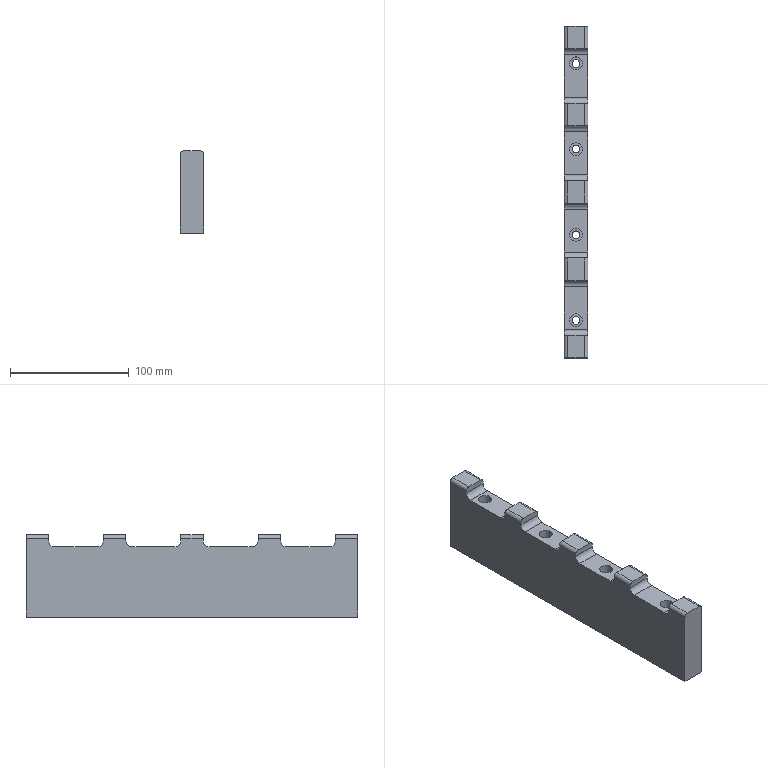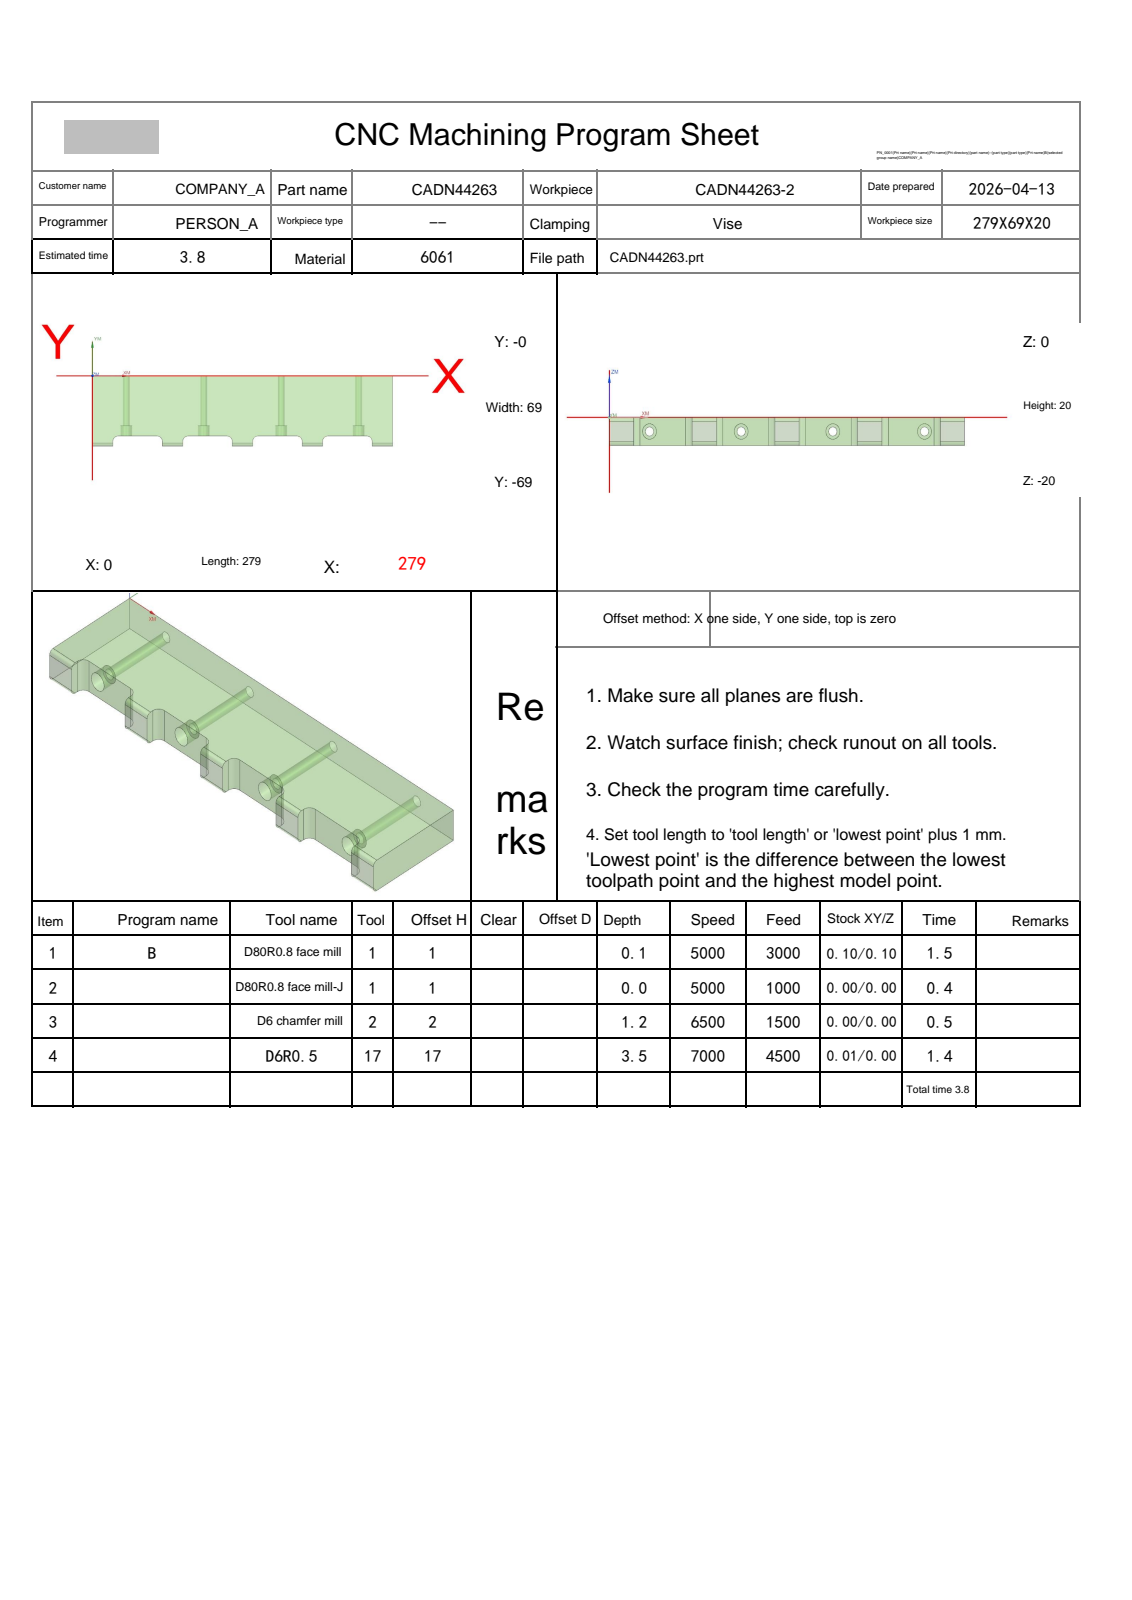NC program | NX | posted by the shop | part box 20 x 279 x 69 mm
Whole program:
%
O0001
(Machine time: 4.53 MIN)
(===Total Tool:3===)
(T1=D80R0.8 face mill D=80.  R=0.8  D-  H01 Z=0.    )
(T2=D6 chamfer mill   D=6.   R=0.   D-  H02 Z=-1.2  )
(T17=D6R0.5 D=6.   R=0.5  D-  H17 Z=-3.5  )
G80 G90 G17 G49 G40
G91 G28 Z0
M01
N1 T01 M06
(D80R0.8 face mill  D=80. R=0.8 H=01 ce=0.10 di=0.10)
G00 G90 G54 X-52.097 Y-34.5 M03 S5000
G43 H01 Z50.
M08
Z6.011
G01 Z4.011 F3000.
X-40.097
X319.097
X331.097
Z6.011
G00 X-52.097
Z5.522
G01 Z3.522
X-40.097
X319.097
X331.097
Z5.522
G00 X-52.097
Z5.033
G01 Z3.033
X-40.097
X319.097
X331.097
Z5.033
G00 X-52.097
Z4.544
G01 Z2.544
X-40.097
X319.097
X331.097
Z4.544
G00 Z50.
X-52.097
Z4.056
G01 Z2.056
X-40.097
X319.097
X331.097
Z4.056
G00 Z50.
X-52.097
Z3.567
G01 Z1.567
X-40.097
X319.097
X331.097
Z3.567
G00 Z50.
X-52.097
Z3.078
G01 Z1.078
X-40.097
X319.097
X331.097
Z3.078
G00 Z50.
X-52.097
Z2.589
G01 Z.589
X-40.097
X319.097
X331.097
Z2.589
G00 Z50.
X-52.097
Z2.1
G01 Z.1
X-40.097
X319.097
X331.097
Z2.1
G00 Z50.
G91 G28 Z0.0
M05
M09
G91 G28 Z0.0
M01
N2 T01 M06
(D80R0.8 face mill-J  D=80. R=0.8 H=01 ce=0.00 di=0.00)
G00 G90 G54 X-51.999 Y-34.5 M03 S5000
G43 H01 Z50.
M08
Z2.
G01 Z0.0 F1000.
X-39.999
X318.999
X330.999
Z2.
G00 Z50.
G91 G28 Z0.0
M05
M09
G91 G28 Z0.0
M01
N3 T02 M06
(D6 chamfer mill  D=6. R=0. H=02 ce=0.00 di=0.00)
G00 G90 G54 X64.072 Y-66.349 M03 S6500
G43 H02 Z50.
M08
Z2.801
G01 Z-1.199 F1500.
X64.034 Y-66.259
X64. Y-66.
Y-64.
G03 X60. Y-60. I-4. J0.0
G01 X24.
G03 X20. Y-64. I0.0 J-4.
G01 Y-66.
X19.997 Y-66.054
X20.027 Y-66.1
G03 X20.227 Y-66.386 I1.732 J1.
G01 Z.145
G00 Z10.
X129.072 Y-66.349
Z2.801
G01 Z-1.199
X129.034 Y-66.259
X129. Y-66.
Y-64.
G03 X125. Y-60. I-4. J0.0
G01 X89.
G03 X85. Y-64. I0.0 J-4.
G01 Y-66.
X84.997 Y-66.054
X85.027 Y-66.1
G03 X85.227 Y-66.386 I1.732 J1.
G01 Z.145
G00 Z10.
X193.773
Z.145
G01 Z-1.199
G03 X193.973 Y-66.1 I-1.532 J1.286
G01 X194.003 Y-66.054
X194. Y-66.
Y-64.
G03 X190. Y-60. I-4. J0.0
G01 X154.
G03 X150. Y-64. I0.0 J-4.
G01 Y-66.
X149.997 Y-66.054
X150.027 Y-66.1
G03 X150.227 Y-66.386 I1.732 J1.
G01 Z.145
G00 Z10.
X258.773
Z.145
G01 Z-1.199
G03 X258.973 Y-66.1 I-1.532 J1.286
G01 X259.003 Y-66.054
X259. Y-66.
Y-64.
G03 X255. Y-60. I-4. J0.0
G01 X219.
G03 X215. Y-64. I0.0 J-4.
G01 Y-66.
X214.997 Y-66.054
X215.027 Y-66.1
G03 X215.227 Y-66.386 I1.732 J1.
G01 Z.145
G00 Z10.
X-1.227
Z.145
G01 Z-1.199
G03 X-1.027 Y-66.1 I-1.532 J1.286
G01 X-.997 Y-66.054
X-1. Y-66.
Y0.0
G02 X0.0 Y1. I1. J0.0
G01 X279.
G02 X280. Y0.0 I0.0 J-1.
G01 Y-66.
X279.997 Y-66.054
X280.027 Y-66.1
G03 X280.227 Y-66.386 I1.732 J1.
G01 Z.145
G00 Z50.
G91 G28 Z0.0
M05
M09
G91 G28 Z0.0
M01
N4 T17 M06
(D6R0.5  D=6. R=0.5 H=17 ce=0.01 di=0.00)
G00 G90 G54 X285.345 Y-67.925 M03 S7000
G43 H17 Z14.8
M08
Z.493
G01 Z-.007 F4500.
X280.1 Y-68.533
X279. Y-68.738
X260.
G03 X259.218 Y-68.576 I-.782 J-1.81
X258.898 Y-68.602 I0.0 J-1.972
G01 X258.9 Y-68.67 Z-.015
G02 X260. Y-68.833 I-.342 J-6.077
G01 X279.
G03 X280.1 Y-68.642 I-.357 J5.306
G01 Y-68.755 Z-.023
X279. Y-68.91
X260.
X259.03 Y-68.74
X258.9 Y-68.731
Y-68.792 Z-.032
X260. Y-68.979
X279.
G02 X280.1 Y-68.813 I20.613 J-132.954
G01 Y-68.861 Z-.037
Y-68.876 Z-.042
X279. Y-69.053
X260.
X258.9 Y-68.85
X258.899 Y-68.898 Z-.049
Y-68.918 Z-.055
G03 X260. Y-69.128 I2.405 J9.652
G01 X279.
X280.1 Y-68.948
Y-69.007 Z-.062
Y-69.031 Z-.069
X279. Y-69.203
X260.
G02 X258.899 Y-68.996 I1.051 J8.641
G01 Y-69.042 Z-.077
Y-69.084 Z-.086
X260. Y-69.279
X279.
X280.1 Y-69.12
Y-69.155 Z-.095
Y-69.188 Z-.104
X279. Y-69.357
X260.
X258.9 Y-69.163
Y-69.196 Z-.114
Y-69.246 Z-.125
X260. Y-69.437
X279.
X279.053 Y-69.433
X280.1 Y-69.267
Y-69.311 Z-.137
Y-69.354 Z-.148
X279. Y-69.518
X260.
G02 X258.9 Y-69.339 I2.137 J16.607
G01 Y-69.386 Z-.161
Y-69.441 Z-.174
G03 X260. Y-69.599 I4.317 J26.016
G01 X279.
X280.1 Y-69.449
Y-69.503 Z-.188
X280.101 Y-69.546 Z-.203
G02 X279. Y-69.684 I-24.833 J193.175
G01 X260.
G02 X258.9 Y-69.541 I4.785 J41.204
G01 Y-69.595 Z-.219
Y-69.642 Z-.235
X260. Y-69.77
X279.
G02 X280.101 Y-69.644 I2.054 J-13.021
G01 Y-69.686 Z-.252
Y-69.727 Z-.269
G02 X279. Y-69.856 I-13.879 J113.455
G01 X260.
X258.9 Y-69.725
Y-69.772 Z-.288
Y-69.814 Z-.306
X260. Y-69.942
X279.
G02 X280.1 Y-69.814 I2.624 J-17.885
G01 Y-69.854 Z-.321
Y-69.883 Z-.337
G03 X279. Y-70.007 I.984 J-13.603
G01 X260.
G02 X258.9 Y-69.884 I3.105 J32.646
G01 Y-69.936 Z-.355
Y-69.97 Z-.374
G02 X260. Y-70.084 I-10.94 J-110.729
G01 X279.
G02 X280.1 Y-69.967 I1.926 J-12.88
G01 Y-70.032 Z-.396
Y-70.067 Z-.418
G03 X279. Y-70.169 I.819 J-14.766
G01 X260.
G03 X258.9 Y-70.066 I-2.92 J-25.349
G01 Y-70.119 Z-.442
Y-70.16 Z-.465
X259.082 Y-70.162
X260. Y-70.253
X279.
G02 X280.1 Y-70.161 I1.249 J-8.298
G01 Y-70.202 Z-.49
Y-70.242 Z-.515
G03 X279. Y-70.337 I.124 J-7.861
G01 X260.
X259.082 Y-70.243
X258.9 Y-70.24
Y-70.285 Z-.54
Y-70.324 Z-.566
X259.082 Y-70.327
X260. Y-70.418
X279.
G02 X280.1 Y-70.326 I1.273 J-8.566
G01 Y-70.368 Z-.591
Y-70.409 Z-.617
X279.742 Y-70.41
G02 X279. Y-70.495 I-.89 J4.508
G01 X260.
G03 X258.9 Y-70.407 I-1.859 J-16.484
G01 Y-70.453 Z-.644
Y-70.489 Z-.67
X259.082 Y-70.491
X260. Y-70.569
X279.
G02 X280.1 Y-70.49 I1.178 J-8.684
G01 Y-70.537 Z-.699
Y-70.563 Z-.729
G03 X279. Y-70.648 I.05 J-7.856
G01 X260.
X259.082 Y-70.564
X258.9 Y-70.562
Y-70.614 Z-.759
Y-70.638 Z-.79
X259.082 Y-70.64
X260. Y-70.725
X279.
G02 X280.1 Y-70.639 I1.177 J-8.027
G01 Y-70.687 Z-.822
Y-70.718 Z-.853
G03 X279. Y-70.8 I.177 J-9.805
G01 X260.
G03 X258.9 Y-70.716 I-1.551 J-13.131
G01 Y-70.763 Z-.886
Y-70.798 Z-.919
G02 X260. Y-70.874 I-.529 J-15.689
G01 X279.
G02 X280.1 Y-70.8 I1.318 J-11.377
G01 Y-70.841 Z-.952
Y-70.876 Z-.986
G03 X279. Y-70.945 I.124 J-10.694
G01 X260.
G03 X258.9 Y-70.874 I-1.437 J-13.654
G01 Y-70.921 Z-1.021
Y-70.951 Z-1.056
X259.082 Y-70.954
X260. Y-71.015
X279.
G02 X280.101 Y-70.953 I1.228 J-11.902
G01 Y-70.989 Z-1.092
Y-71.021 Z-1.128
G03 X279. Y-71.084 I.035 J-10.406
G01 X260.
G03 X258.9 Y-71.02 I-1.26 J-12.225
G01 Y-71.054 Z-1.165
Y-71.083 Z-1.202
X259.427 Y-71.096
G03 X260. Y-71.15 I.614 J3.478
G01 X279.
G02 X280.1 Y-71.085 I1.194 J-10.827
G01 Y-71.118 Z-1.24
Y-71.149 Z-1.278
G03 X279. Y-71.214 I.089 J-10.915
G01 X260.
G02 X259.427 Y-71.161 I.105 J4.261
G01 X258.9 Y-71.148
Y-71.183 Z-1.316
Y-71.212 Z-1.355
G02 X260. Y-71.276 I-.313 J-14.825
G01 X279.
G02 X280.1 Y-71.213 I1.165 J-10.805
G01 X280.101 Y-71.25 Z-1.395
Y-71.279 Z-1.434
G03 X279. Y-71.336 I.103 J-12.677
G01 X260.
G03 X258.9 Y-71.277 I-1.704 J-21.57
G01 Y-71.31 Z-1.475
Y-71.339 Z-1.516
G02 X260. Y-71.393 I-.086 J-12.93
G01 X279.
G02 X280.08 Y-71.34 I1.08 J-11.01
G01 X280.101
Y-71.367 Z-1.557
Y-71.391 Z-1.598
X280.085
G03 X279. Y-71.448 I0.0 J-10.303
G01 X260.
X259.427 Y-71.4
X258.9 Y-71.39
Y-71.418 Z-1.641
Y-71.441 Z-1.683
X259.427 Y-71.452
G03 X260. Y-71.501 I.616 J3.827
G01 X279.
X279.053 Y-71.5
X279.727 Y-71.446
G02 X279.938 Y-71.438 I.211 J-2.639
G01 X280.1 Y-71.443
Y-71.47 Z-1.726
Y-71.496 Z-1.769
X280.052
G03 X279. Y-71.552 I0.0 J-9.962
G01 X260.
G02 X259.427 Y-71.505 I.274 J6.879
G01 X258.9 Y-71.496
Y-71.523 Z-1.812
Y-71.547 Z-1.856
G02 X260. Y-71.6 I-.079 J-13.17
G01 X279.
G02 X279.98 Y-71.548 I.98 J-9.242
G01 X280.101 Y-71.549
Y-71.573 Z-1.9
Y-71.597 Z-1.945
X279.972 Y-71.596
G03 X279. Y-71.645 I0.0 J-9.55
G01 X260.
G03 X258.9 Y-71.596 I-1.189 J-14.048
G01 Y-71.618 Z-1.99
Y-71.635 Z-2.035
X259.427 Y-71.644
G03 X260. Y-71.689 I.669 J4.914
G01 X279.
G02 X280.09 Y-71.636 I1.09 J-11.268
G01 X280.101
Y-71.657 Z-2.08
Y-71.675 Z-2.126
X280.025
G03 X279. Y-71.729 I0.0 J-9.733
G01 X260.
G02 X259.427 Y-71.683 I.123 J5.164
G01 X258.9 Y-71.674
Y-71.695 Z-2.172
Y-71.712 Z-2.218
X259.427 Y-71.722
G03 X260. Y-71.767 I.648 J4.552
G01 X279.
G02 X279.983 Y-71.713 I.983 J-8.893
G01 X280.101 Y-71.714
Y-71.734 Z-2.265
Y-71.752 Z-2.312
X279.959 Y-71.751
G03 X279. Y-71.802 I0.0 J-9.028
G01 X260.
G02 X259.427 Y-71.76 I.241 J7.253
G01 X258.9 Y-71.751
Y-71.771 Z-2.359
Y-71.789 Z-2.406
G02 X260. Y-71.835 I-.203 J-18.176
G01 X279.
G02 X279.96 Y-71.79 I.96 J-10.236
G01 X280.102 Y-71.791
X280.101 Y-71.807 Z-2.454
X280.1 Y-71.817 Z-2.502
X280.092
G03 X279. Y-71.865 I0.0 J-12.564
G01 X260.
X259.427 Y-71.824
X258.9 Y-71.817
X258.898 Y-71.833 Z-2.55
X258.896 Y-71.846 Z-2.598
X259.427 Y-71.85
X260. Y-71.892
X279.
G02 X280.038 Y-71.842 I1.038 J-10.908
G01 X280.1 Y-71.843
X280.097 Y-71.854 Z-2.646
X280.095 Y-71.866 Z-2.695
G03 X279. Y-71.916 I.01 J-12.239
G01 X260.
X259.427 Y-71.875
X258.896 Y-71.872
Y-71.885 Z-2.744
X258.895 Y-71.898 Z-2.792
X259.427 Y-71.901
X260. Y-71.938
X279.
G02 X280.096 Y-71.89 I1.259 J-16.152
G01 X280.097 Y-71.901 Z-2.841
Y-71.913 Z-2.891
G03 X279. Y-71.957 I.411 J-24.268
G01 X260.
G03 X258.995 Y-71.922 I-1.005 J-14.556
G01 X258.895
Y-71.931 Z-2.94
Y-71.942 Z-2.989
X259.028 Y-71.941
G02 X260. Y-71.973 I0.0 J-15.169
G01 X279.
G02 X280.098 Y-71.935 I1.532 J-29.007
G01 X280.099 Y-71.945 Z-3.039
Y-71.955 Z-3.088
X279. Y-71.986
X260.
G03 X259.128 Y-71.96 I-.872 J-14.727
X258.895 Y-71.962 I0.0 J-14.753
G01 X258.905 Y-71.976 Z-3.188
G02 X259.203 Y-71.973 I.298 J-13.938
X260. Y-71.996 I0.0 J-13.941
G01 X279.
X279.053 Y-71.993
X280.1 Y-71.973
X280.101 Y-71.979 Z-3.227
Y-71.983 Z-3.266
X279.053 Y-71.998
X279. Y-72.002
X260.
G03 X259.208 Y-71.983 I-.792 J-16.081
X258.905 Y-71.986 I0.0 J-16.1
G01 Y-71.995 Z-3.344
G02 X259.211 Y-71.992 I.306 J-22.158
X260. Y-72.007 I0.0 J-22.16
G01 X279.
X280.101 Y-71.993
X280.102 Y-71.999 Z-3.383
Y-72.003 Z-3.422
X279. Y-72.009
X260.
X258.905 Y-72.004
Y-72.009 Z-3.5
X280.102
G00 Z14.8
X219.775 Y-69.035
Z.493
G01 Z-.007
X215.1 Y-68.532
X214.882 Y-68.533
X214. Y-68.738
X195.
X194.118 Y-68.533
X193.91 Y-68.573
X193.903 Y-68.638 Z-.011
X193.902 Y-68.651 Z-.015
X194.81 Y-68.807
X195. Y-68.833
X214.
G02 X215.1 Y-68.64 I11.736 J-63.511
G01 Y-68.721 Z-.019
Y-68.752 Z-.023
X214. Y-68.91
X195.
X193.898 Y-68.732
X193.9 Y-68.79 Z-.032
X194.113 Y-68.818
X195. Y-68.979
X214.
X214.882 Y-68.813
X215.1 Y-68.812
Y-68.861 Z-.037
Y-68.875 Z-.042
X214.882 Y-68.877
X214. Y-69.053
X195.
X194.109 Y-68.893
X193.9 Y-68.847
Y-68.898 Z-.049
Y-68.915 Z-.055
X194.096 Y-68.955
X195. Y-69.128
X214.
X214.882 Y-68.951
X215.1 Y-68.948
Y-69.007 Z-.062
Y-69.031 Z-.069
X214. Y-69.203
X195.
G02 X193.9 Y-68.992 I1.243 J9.475
G01 Y-69.043 Z-.077
Y-69.081 Z-.086
X194.066 Y-69.107
X195. Y-69.279
X214.
X215.1 Y-69.12
Y-69.155 Z-.095
Y-69.189 Z-.104
X214. Y-69.357
X195.
X193.899 Y-69.164
Y-69.196 Z-.114
Y-69.248 Z-.125
X195. Y-69.437
X214.
X215.1 Y-69.268
Y-69.311 Z-.137
Y-69.355 Z-.148
X214. Y-69.518
X195.
X194.81 Y-69.503
X193.9 Y-69.342
Y-69.386 Z-.161
Y-69.441 Z-.174
X195. Y-69.599
X214.
X215.1 Y-69.45
Y-69.503 Z-.188
Y-69.546 Z-.203
X214.882 Y-69.55
X214. Y-69.684
X195.
X194.118 Y-69.55
X193.899 Y-69.543
X193.9 Y-69.596 Z-.219
Y-69.643 Z-.235
X195. Y-69.77
X214.
X214.882 Y-69.645
X215.1 Y-69.643
Y-69.686 Z-.252
Y-69.726 Z-.269
X214.882 Y-69.728
X214. Y-69.856
X195.
X193.9 Y-69.726
Y-69.772 Z-.288
Y-69.813 Z-.306
X194.118 Y-69.815
X195. Y-69.942
X214.
X214.882 Y-69.817
X215.1 Y-69.814
Y-69.854 Z-.321
Y-69.884 Z-.337
G03 X214. Y-70.007 I11.318 J-105.893
G01 X195.
X194.118 Y-69.884
X193.9 Y-69.882
Y-69.936 Z-.355
Y-69.966 Z-.374
X195. Y-70.084
X214.
X214.882 Y-69.978
X215.1 Y-69.97
Y-70.033 Z-.396
Y-70.067 Z-.418
X214.882 Y-70.072
X214. Y-70.169
X195.
X193.9 Y-70.065
Y-70.119 Z-.442
Y-70.16 Z-.465
X194.118 Y-70.162
X195. Y-70.253
X214.
X214.882 Y-70.162
X215.1 Y-70.16
Y-70.202 Z-.49
Y-70.241 Z-.515
X214.882 Y-70.243
X214. Y-70.337
X195.
G02 X194.292 Y-70.247 I.042 J3.181
G01 X193.9 Y-70.241
Y-70.285 Z-.54
Y-70.325 Z-.566
X194.118 Y-70.327
X195. Y-70.418
X214.
X214.882 Y-70.327
X215.1 Y-70.325
Y-70.368 Z-.591
Y-70.408 Z-.617
X214.882 Y-70.41
X214. Y-70.495
X195.
X193.9 Y-70.408
Y-70.453 Z-.644
Y-70.49 Z-.67
X194.118 Y-70.491
X195. Y-70.569
X214.
G02 X215.1 Y-70.49 I1.409 J-11.774
G01 Y-70.537 Z-.699
Y-70.563 Z-.729
G03 X214. Y-70.648 I.234 J-10.139
G01 X195.
X194.118 Y-70.564
X193.9 Y-70.563
Y-70.614 Z-.759
Y-70.638 Z-.79
X194.118 Y-70.64
X195. Y-70.725
X214.
G02 X215.1 Y-70.638 I1.321 J-9.774
G01 Y-70.687 Z-.822
Y-70.717 Z-.853
X214.955 Y-70.709
X214.821 Y-70.716
X214. Y-70.8
X195.
X194.118 Y-70.719
X193.9 Y-70.717
Y-70.763 Z-.886
Y-70.798 Z-.919
X194.118 Y-70.8
X195. Y-70.874
X214.
X214.536 Y-70.823
X214.62 Y-70.814
X215.1 Y-70.798
Y-70.841 Z-.952
Y-70.875 Z-.986
X214.882 Y-70.877
X214. Y-70.945
X195.
X194.118 Y-70.877
X193.9 Y-70.875
Y-70.919 Z-1.021
Y-70.952 Z-1.056
X194.118 Y-70.954
X195. Y-71.015
X214.
X214.882 Y-70.954
X215.1 Y-70.952
Y-70.989 Z-1.092
Y-71.021 Z-1.128
G03 X214. Y-71.084 I.106 J-11.464
G01 X195.
G03 X193.9 Y-71.021 I-1.206 J-11.401
G01 Y-71.054 Z-1.165
Y-71.084 Z-1.202
X194.464 Y-71.1
G03 X195. Y-71.15 I.558 J3.082
G01 X214.
G03 X214.536 Y-71.1 I-.021 J3.132
G01 X215.1 Y-71.084
Y-71.118 Z-1.24
Y-71.148 Z-1.278
G03 X214. Y-71.214 I.353 J-15.186
G01 X195.
G03 X193.9 Y-71.148 I-1.453 J-15.12
G01 Y-71.183 Z-1.316
Y-71.212 Z-1.355
G02 X195. Y-71.276 I-.249 J-13.86
G01 X214.
G02 X215.1 Y-71.212 I1.349 J-13.797
G01 Y-71.25 Z-1.395
Y-71.277 Z-1.434
G03 X214. Y-71.336 I.651 J-22.793
G01 X195.
G03 X193.9 Y-71.277 I-1.752 J-22.735
G01 Y-71.31 Z-1.475
Y-71.339 Z-1.516
G02 X195. Y-71.393 I-.06 J-12.531
G01 X214.
G02 X215.1 Y-71.339 I1.16 J-12.478
G01 Y-71.367 Z-1.557
Y-71.39 Z-1.598
G03 X214. Y-71.448 I.169 J-13.623
G01 X195.
G03 X193.9 Y-71.39 I-1.269 J-13.564
G01 Y-71.418 Z-1.641
Y-71.442 Z-1.683
X194.464 Y-71.455
G03 X195. Y-71.501 I.55 J3.271
G01 X214.
G03 X214.536 Y-71.455 I-.02 J3.386
G01 X215.1 Y-71.442
Y-71.47 Z-1.726
Y-71.496 Z-1.769
G03 X214. Y-71.552 I.175 J-14.347
G01 X195.
G03 X193.9 Y-71.496 I-1.275 J-14.292
G01 Y-71.523 Z-1.812
Y-71.548 Z-1.856
G02 X195. Y-71.6 I-.069 J-13.12
G01 X214.
G02 X215.1 Y-71.548 I1.169 J-13.068
G01 Y-71.573 Z-1.9
Y-71.596 Z-1.945
G03 X214. Y-71.645 I.103 J-14.555
G01 X195.
G03 X193.9 Y-71.596 I-1.203 J-14.506
G01 Y-71.618 Z-1.99
Y-71.635 Z-2.035
X194.464 Y-71.647
G03 X195. Y-71.689 I.605 J4.327
G01 X214.
G03 X214.536 Y-71.647 I-.069 J4.369
G01 X215.1 Y-71.635
Y-71.657 Z-2.08
Y-71.674 Z-2.126
X214.536 Y-71.686
G02 X214. Y-71.729 I-.622 J4.418
G01 X195.
G02 X194.464 Y-71.686 I.086 J4.461
G01 X193.9 Y-71.674
Y-71.695 Z-2.172
Y-71.713 Z-2.218
X194.464 Y-71.725
G03 X195. Y-71.767 I.59 J4.056
G01 X214.
G03 X214.536 Y-71.725 I-.054 J4.098
G01 X215.1 Y-71.713
Y-71.734 Z-2.265
Y-71.751 Z-2.312
X214.536 Y-71.761
G02 X214. Y-71.802 I-.689 J5.53
G01 X195.
G02 X194.464 Y-71.763 I.182 J6.232
G01 X193.9 Y-71.751
Y-71.771 Z-2.359
Y-71.79 Z-2.406
X194.464 Y-71.8
G03 X195. Y-71.835 I.669 J6.159
G01 X214.
X214.19 Y-71.828
G02 X214.861 Y-71.784 I.671 J-5.154
X215.1 Y-71.79 I0.0 J-5.198
G01 Y-71.807 Z-2.454
Y-71.816 Z-2.502
G03 X214. Y-71.865 I.147 J-15.87
G01 X195.
G03 X193.9 Y-71.818 I-1.19 J-15.04
G01 X193.898 Y-71.833 Z-2.55
X193.897 Y-71.846 Z-2.598
X193.953
G02 X195. Y-71.892 I0.0 J-12.019
G01 X214.
G02 X215.103 Y-71.843 I1.135 J-13.09
G01 Y-71.854 Z-2.646
Y-71.866 Z-2.695
G03 X214. Y-71.916 I.267 J-18.114
G01 X195.
G02 X194.464 Y-71.878 I.19 J6.461
G01 X193.897 Y-71.872
Y-71.885 Z-2.744
Y-71.898 Z-2.792
X194.464 Y-71.903
X195. Y-71.938
X214.
G02 X215.103 Y-71.89 I1.534 J-22.69
G01 Y-71.901 Z-2.841
Y-71.914 Z-2.891
G03 X214. Y-71.957 I.475 J-26.586
G01 X195.
G03 X194.065 Y-71.923 I-.935 J-13.098
G01 X193.897 Y-71.924
Y-71.931 Z-2.94
X193.896 Y-71.943 Z-2.989
X194.071 Y-71.942
G02 X195. Y-71.973 I0.0 J-14.242
G01 X214.
G02 X215.103 Y-71.935 I1.619 J-31.516
G01 X215.104 Y-71.944 Z-3.039
Y-71.955 Z-3.088
X214.19 Y-71.976
X214. Y-71.986
X195.
G03 X194.142 Y-71.96 I-.858 J-14.468
X193.896 Y-71.962 I0.0 J-14.494
G01 Y-71.966 Z-3.138
Y-71.976 Z-3.188
X194.81 Y-71.984
X195. Y-71.996
X214.
X214.19 Y-71.984
X215.104 Y-71.972
Y-71.979 Z-3.227
Y-71.982 Z-3.266
X214.19 Y-71.991
X214. Y-72.002
X195.
X194.81 Y-71.991
X193.896 Y-71.985
Y-71.994 Z-3.344
X194.81 Y-71.998
X195. Y-72.007
X214.
X214.19 Y-71.998
X215.104 Y-71.992
Y-71.998 Z-3.383
Y-72.003 Z-3.422
X214.19 Y-72.005
X214. Y-72.009
X195.
X194.81 Y-72.005
X193.896 Y-72.003
Y-72.009 Z-3.5
X215.104
G00 Z14.8
X154.771 Y-69.038
Z.493
G01 Z-.007
X150.1 Y-68.532
X149.884
X149. Y-68.738
X130.
X129.116 Y-68.532
X128.91 Y-68.572
X128.903 Y-68.638 Z-.011
X128.902 Y-68.651 Z-.015
G02 X130. Y-68.833 I-3.049 J-21.763
G01 X149.
G02 X150.1 Y-68.64 I11.734 J-63.449
G01 Y-68.721 Z-.019
Y-68.753 Z-.023
X149. Y-68.91
X130.
X128.898 Y-68.732
X128.9 Y-68.79 Z-.032
X129.111 Y-68.818
X130. Y-68.979
X149.
X149.884 Y-68.813
X150.1 Y-68.812
Y-68.861 Z-.037
Y-68.874 Z-.042
X149.884 Y-68.876
X149. Y-69.053
X130.
X129.108 Y-68.892
X128.9 Y-68.848
Y-68.898 Z-.049
Y-68.916 Z-.055
X129.095 Y-68.955
X130. Y-69.128
X149.
X149.884 Y-68.95
X150.1 Y-68.948
Y-69.007 Z-.062
Y-69.031 Z-.069
X149. Y-69.203
X130.
G02 X128.9 Y-68.994 I.939 J7.967
G01 Y-69.042 Z-.077
Y-69.084 Z-.086
X129.064 Y-69.106
X130. Y-69.279
X149.
X150.1 Y-69.119
Y-69.155 Z-.095
Y-69.189 Z-.104
X149. Y-69.357
X130.
X128.899 Y-69.164
Y-69.196 Z-.114
Y-69.248 Z-.125
X130. Y-69.437
X149.
X150.1 Y-69.267
Y-69.311 Z-.137
Y-69.355 Z-.148
X149. Y-69.518
X130.
X129.808 Y-69.503
X128.9 Y-69.342
Y-69.386 Z-.161
Y-69.441 Z-.174
X130. Y-69.599
X149.
X150.1 Y-69.45
Y-69.503 Z-.188
Y-69.546 Z-.203
X149.884 Y-69.55
X149. Y-69.684
X130.
X129.116 Y-69.55
X128.9 Y-69.543
Y-69.596 Z-.219
Y-69.643 Z-.235
X130. Y-69.77
X149.
X149.884 Y-69.645
X150.1 Y-69.643
Y-69.686 Z-.252
Y-69.726 Z-.269
X149.884 Y-69.728
X149. Y-69.856
X130.
X128.9 Y-69.726
Y-69.772 Z-.288
Y-69.813 Z-.306
X129.116 Y-69.815
X130. Y-69.942
X149.
X149.884 Y-69.817
X150.1 Y-69.814
Y-69.854 Z-.321
Y-69.884 Z-.337
G03 X149. Y-70.007 I11.328 J-105.982
G01 X130.
X129.116 Y-69.884
X128.9 Y-69.882
Y-69.936 Z-.355
Y-69.966 Z-.374
X130. Y-70.084
X149.
X149.884 Y-69.978
X150.1 Y-69.97
Y-70.032 Z-.396
Y-70.067 Z-.418
X149.884 Y-70.072
X149. Y-70.169
X130.
X128.9 Y-70.066
Y-70.119 Z-.442
Y-70.16 Z-.465
X129.116 Y-70.162
X130. Y-70.253
X149.
X149.884 Y-70.162
X150.1 Y-70.16
Y-70.202 Z-.49
Y-70.241 Z-.515
X149.884 Y-70.243
X149. Y-70.337
X130.
G02 X129.291 Y-70.247 I.043 J3.197
G01 X128.9 Y-70.241
Y-70.285 Z-.54
Y-70.325 Z-.566
X129.116 Y-70.327
X130. Y-70.418
X149.
X149.884 Y-70.327
X150.1 Y-70.325
Y-70.368 Z-.591
Y-70.408 Z-.617
X149.884 Y-70.41
X149. Y-70.495
X130.
X128.9 Y-70.408
Y-70.453 Z-.644
Y-70.489 Z-.67
X129.116 Y-70.491
X130. Y-70.569
X149.
G02 X150.1 Y-70.489 I1.413 J-11.804
G01 Y-70.537 Z-.699
Y-70.562 Z-.729
G03 X149. Y-70.648 I.236 J-10.157
G01 X130.
X129.116 Y-70.564
X128.9 Y-70.562
Y-70.614 Z-.759
Y-70.638 Z-.79
X129.116 Y-70.64
X130. Y-70.725
X149.
G02 X150.1 Y-70.638 I1.324 J-9.805
G01 Y-70.687 Z-.822
Y-70.717 Z-.853
X149.956 Y-70.711
X149.784 Y-70.72
X149. Y-70.8
X130.
X129.116 Y-70.719
X128.9 Y-70.717
Y-70.763 Z-.886
Y-70.798 Z-.919
X129.116 Y-70.8
X130. Y-70.874
X149.
X149.538 Y-70.822
X149.626 Y-70.813
X150.1 Y-70.798
Y-70.841 Z-.952
Y-70.875 Z-.986
X149.884 Y-70.877
X149. Y-70.945
X130.
X129.116 Y-70.877
X128.9 Y-70.875
Y-70.921 Z-1.021
Y-70.952 Z-1.056
X129.116 Y-70.954
X130. Y-71.015
X149.
X149.884 Y-70.954
X150.1 Y-70.952
Y-70.989 Z-1.092
Y-71.02 Z-1.128
G03 X149. Y-71.084 I.108 J-11.494
G01 X130.
G03 X128.9 Y-71.02 I-1.208 J-11.431
G01 Y-71.054 Z-1.165
Y-71.084 Z-1.202
X129.462 Y-71.1
G03 X130. Y-71.15 I.559 J3.085
G01 X149.
G03 X149.538 Y-71.1 I-.021 J3.135
G01 X150.1 Y-71.084
Y-71.118 Z-1.24
Y-71.148 Z-1.278
G03 X149. Y-71.214 I.356 J-15.218
G01 X130.
G03 X128.9 Y-71.148 I-1.456 J-15.152
G01 Y-71.183 Z-1.316
Y-71.212 Z-1.355
G02 X130. Y-71.276 I-.253 J-13.932
G01 X149.
G02 X150.1 Y-71.212 I1.353 J-13.869
G01 Y-71.25 Z-1.395
Y-71.278 Z-1.434
G03 X149. Y-71.336 I.659 J-22.96
G01 X130.
G03 X128.9 Y-71.278 I-1.759 J-22.9
G01 Y-71.31 Z-1.475
Y-71.339 Z-1.516
G02 X130. Y-71.393 I-.061 J-12.531
G01 X149.
G02 X150.1 Y-71.339 I1.161 J-12.477
G01 Y-71.367 Z-1.557
Y-71.39 Z-1.598
G03 X149. Y-71.448 I.174 J-13.705
G01 X130.
G03 X128.9 Y-71.39 I-1.274 J-13.647
G01 Y-71.418 Z-1.641
Y-71.442 Z-1.683
X129.462 Y-71.455
G03 X130. Y-71.501 I.551 J3.272
G01 X149.
G03 X149.538 Y-71.455 I-.017 J3.362
G01 X150.1 Y-71.442
Y-71.47 Z-1.726
Y-71.496 Z-1.769
G03 X149. Y-71.552 I.189 J-14.504
G01 X130.
G03 X128.9 Y-71.496 I-1.288 J-14.447
G01 Y-71.523 Z-1.812
Y-71.548 Z-1.856
G02 X130. Y-71.6 I-.07 J-13.129
G01 X149.
G02 X150.1 Y-71.548 I1.17 J-13.077
G01 Y-71.573 Z-1.9
Y-71.596 Z-1.945
G03 X149. Y-71.645 I.111 J-14.702
G01 X130.
G03 X128.9 Y-71.596 I-1.211 J-14.652
G01 Y-71.618 Z-1.99
Y-71.635 Z-2.035
X129.462 Y-71.647
G03 X130. Y-71.689 I.608 J4.36
G01 X149.
G03 X149.538 Y-71.647 I-.07 J4.402
G01 X150.1 Y-71.635
Y-71.657 Z-2.08
Y-71.674 Z-2.126
X149.538 Y-71.686
G02 X149. Y-71.729 I-.624 J4.432
G01 X130.
G02 X129.462 Y-71.686 I.086 J4.475
G01 X128.9 Y-71.674
Y-71.695 Z-2.172
Y-71.713 Z-2.218
X129.462 Y-71.724
G03 X130. Y-71.767 I.594 J4.092
G01 X149.
G03 X149.538 Y-71.724 I-.056 J4.134
G01 X150.1 Y-71.713
Y-71.734 Z-2.265
Y-71.751 Z-2.312
X149.538 Y-71.761
G02 X149. Y-71.802 I-.691 J5.54
G01 X130.
G02 X129.462 Y-71.763 I.184 J6.258
G01 X128.9 Y-71.751
Y-71.771 Z-2.359
Y-71.79 Z-2.406
X129.462 Y-71.8
G03 X130. Y-71.835 I.668 J6.118
G01 X149.
X149.192 Y-71.828
G02 X149.86 Y-71.784 I.669 J-5.13
X150.1 Y-71.79 I0.0 J-5.173
G01 Y-71.807 Z-2.454
Y-71.816 Z-2.502
G03 X149. Y-71.865 I.142 J-15.739
G01 X130.
G03 X128.9 Y-71.818 I-1.186 J-14.917
G01 Y-71.833 Z-2.55
Y-71.846 Z-2.598
X128.957
G02 X130. Y-71.892 I0.0 J-11.927
G01 X149.
G02 X150.1 Y-71.843 I1.132 J-13.003
G01 Y-71.854 Z-2.646
Y-71.866 Z-2.695
G03 X149. Y-71.916 I.261 J-17.894
G01 X130.
G02 X129.462 Y-71.878 I.199 J6.597
G01 X128.9 Y-71.872
Y-71.885 Z-2.744
Y-71.898 Z-2.792
X129.462 Y-71.903
G03 X130. Y-71.938 I.695 J6.615
G01 X149.
G02 X150.1 Y-71.89 I1.541 J-22.828
G01 Y-71.902 Z-2.841
Y-71.914 Z-2.891
X149.884 Y-71.918
X149. Y-71.957
X130.
G03 X129.014 Y-71.922 I-.986 J-14.218
G01 X128.901 Y-71.923
X128.9 Y-71.937 Z-2.94
Y-71.943 Z-2.989
X129.072 Y-71.942
G02 X130. Y-71.973 I0.0 J-14.315
G01 X149.
X149.884 Y-71.939
X150.1 Y-71.935
Y-71.945 Z-3.039
Y-71.955 Z-3.088
X149.192 Y-71.975
X149. Y-71.986
X130.
G03 X129.112 Y-71.96 I-.888 J-15.263
X128.9 Y-71.961 I0.0 J-15.289
G01 Y-71.971 Z-3.138
Y-71.975 Z-3.188
X129.808 Y-71.984
X130. Y-71.996
X149.
X149.192 Y-71.984
X150.1 Y-71.971
Y-71.979 Z-3.227
Y-71.982 Z-3.266
X149.192 Y-71.991
X149. Y-72.002
X130.
X129.808 Y-71.99
X128.9 Y-71.986
X128.905 Y-71.995 Z-3.344
X128.911 Y-71.993
X129.808 Y-71.997
X130. Y-72.007
X149.
X149.192 Y-71.997
X150.089 Y-71.992
X150.1 Y-71.994
X150.095 Y-72.002 Z-3.422
X149.192 Y-72.004
X149. Y-72.009
X130.
X129.808 Y-72.004
X128.905 Y-72.003
Y-72.01 Z-3.5
X150.095
G00 Z14.8
X89.775 Y-69.035
Z.493
G01 Z-.007
X85.1 Y-68.532
X84.882 Y-68.533
X84. Y-68.738
X65.
X64.118 Y-68.533
X63.91 Y-68.573
X63.903 Y-68.638 Z-.011
X63.902 Y-68.651 Z-.015
X64.81 Y-68.807
X65. Y-68.833
X84.
G02 X85.1 Y-68.64 I11.736 J-63.511
G01 Y-68.721 Z-.019
Y-68.752 Z-.023
X84. Y-68.91
X65.
X63.898 Y-68.732
X63.9 Y-68.79 Z-.032
X64.113 Y-68.818
X65. Y-68.979
X84.
X84.882 Y-68.813
X85.1 Y-68.812
Y-68.861 Z-.037
Y-68.875 Z-.042
X84.882 Y-68.877
X84. Y-69.053
X65.
X64.109 Y-68.893
X63.9 Y-68.847
Y-68.898 Z-.049
Y-68.915 Z-.055
X64.096 Y-68.955
X65. Y-69.128
X84.
X84.882 Y-68.951
X85.1 Y-68.948
Y-69.007 Z-.062
Y-69.031 Z-.069
X84. Y-69.203
X65.
G02 X63.9 Y-68.992 I1.243 J9.475
G01 Y-69.043 Z-.077
Y-69.081 Z-.086
X64.066 Y-69.107
X65. Y-69.279
X84.
X85.1 Y-69.12
Y-69.155 Z-.095
Y-69.189 Z-.104
X84. Y-69.357
X65.
X63.899 Y-69.164
Y-69.196 Z-.114
Y-69.248 Z-.125
X65. Y-69.437
X84.
X85.1 Y-69.268
Y-69.311 Z-.137
Y-69.355 Z-.148
X84. Y-69.518
X65.
X64.81 Y-69.503
X63.9 Y-69.342
Y-69.386 Z-.161
Y-69.441 Z-.174
X65. Y-69.599
X84.
X85.1 Y-69.45
Y-69.503 Z-.188
Y-69.546 Z-.203
X84.882 Y-69.55
X84. Y-69.684
X65.
X64.118 Y-69.55
X63.899 Y-69.543
X63.9 Y-69.596 Z-.219
Y-69.643 Z-.235
X65. Y-69.77
X84.
X84.882 Y-69.645
X85.1 Y-69.643
Y-69.686 Z-.252
Y-69.726 Z-.269
X84.882 Y-69.728
X84. Y-69.856
X65.
X63.9 Y-69.726
Y-69.772 Z-.288
Y-69.813 Z-.306
X64.118 Y-69.815
X65. Y-69.942
X84.
X84.882 Y-69.817
X85.1 Y-69.814
Y-69.854 Z-.321
Y-69.884 Z-.337
G03 X84. Y-70.007 I11.318 J-105.893
G01 X65.
X64.118 Y-69.884
X63.9 Y-69.882
Y-69.936 Z-.355
Y-69.966 Z-.374
X65. Y-70.084
X84.
X84.882 Y-69.978
X85.1 Y-69.97
Y-70.033 Z-.396
Y-70.067 Z-.418
X84.882 Y-70.072
X84. Y-70.169
X65.
X63.9 Y-70.065
Y-70.119 Z-.442
Y-70.16 Z-.465
X64.118 Y-70.162
X65. Y-70.253
X84.
X84.882 Y-70.162
X85.1 Y-70.16
Y-70.202 Z-.49
Y-70.241 Z-.515
X84.882 Y-70.243
X84. Y-70.337
X65.
G02 X64.292 Y-70.247 I.042 J3.181
G01 X63.9 Y-70.241
Y-70.285 Z-.54
Y-70.325 Z-.566
X64.118 Y-70.327
X65. Y-70.418
X84.
X84.882 Y-70.327
X85.1 Y-70.325
Y-70.368 Z-.591
Y-70.408 Z-.617
X84.882 Y-70.41
X84. Y-70.495
X65.
X63.9 Y-70.408
Y-70.453 Z-.644
Y-70.49 Z-.67
X64.118 Y-70.491
X65. Y-70.569
X84.
G02 X85.1 Y-70.49 I1.409 J-11.774
G01 Y-70.537 Z-.699
Y-70.563 Z-.729
G03 X84. Y-70.648 I.234 J-10.139
G01 X65.
X64.118 Y-70.564
X63.9 Y-70.563
Y-70.614 Z-.759
Y-70.638 Z-.79
X64.118 Y-70.64
X65. Y-70.725
X84.
G02 X85.1 Y-70.638 I1.321 J-9.774
G01 Y-70.687 Z-.822
Y-70.717 Z-.853
X84.956 Y-70.711
X84.785 Y-70.72
X84. Y-70.8
X65.
X64.118 Y-70.719
X63.9 Y-70.717
Y-70.763 Z-.886
Y-70.798 Z-.919
X64.118 Y-70.8
X65. Y-70.874
X84.
X84.536 Y-70.823
X84.62 Y-70.814
X85.1 Y-70.798
Y-70.841 Z-.952
Y-70.875 Z-.986
X84.882 Y-70.877
X84. Y-70.945
X65.
X64.118 Y-70.877
X63.9 Y-70.875
Y-70.919 Z-1.021
Y-70.952 Z-1.056
X64.118 Y-70.954
X65. Y-71.015
X84.
X84.882 Y-70.954
X85.1 Y-70.952
Y-70.989 Z-1.092
Y-71.021 Z-1.128
G03 X84. Y-71.084 I.106 J-11.464
G01 X65.
G03 X63.9 Y-71.021 I-1.206 J-11.401
G01 Y-71.054 Z-1.165
Y-71.084 Z-1.202
X64.464 Y-71.1
G03 X65. Y-71.15 I.558 J3.082
G01 X84.
G03 X84.536 Y-71.1 I-.021 J3.132
G01 X85.1 Y-71.084
Y-71.118 Z-1.24
Y-71.148 Z-1.278
G03 X84. Y-71.214 I.353 J-15.186
G01 X65.
G03 X63.9 Y-71.148 I-1.453 J-15.12
G01 Y-71.183 Z-1.316
Y-71.212 Z-1.355
G02 X65. Y-71.276 I-.249 J-13.86
G01 X84.
G02 X85.1 Y-71.212 I1.349 J-13.797
G01 Y-71.25 Z-1.395
Y-71.277 Z-1.434
G03 X84. Y-71.336 I.651 J-22.793
G01 X65.
G03 X63.9 Y-71.277 I-1.752 J-22.735
G01 Y-71.31 Z-1.475
Y-71.339 Z-1.516
G02 X65. Y-71.393 I-.06 J-12.531
G01 X84.
G02 X85.1 Y-71.339 I1.16 J-12.478
G01 Y-71.367 Z-1.557
Y-71.39 Z-1.598
G03 X84. Y-71.448 I.169 J-13.623
G01 X65.
G03 X63.9 Y-71.39 I-1.269 J-13.564
G01 Y-71.418 Z-1.641
Y-71.442 Z-1.683
X64.464 Y-71.455
G03 X65. Y-71.501 I.55 J3.271
G01 X84.
G03 X84.536 Y-71.455 I-.02 J3.386
G01 X85.1 Y-71.442
Y-71.47 Z-1.726
Y-71.496 Z-1.769
G03 X84. Y-71.552 I.175 J-14.347
G01 X65.
G03 X63.9 Y-71.496 I-1.275 J-14.292
G01 Y-71.523 Z-1.812
Y-71.548 Z-1.856
G02 X65. Y-71.6 I-.069 J-13.12
G01 X84.
G02 X85.1 Y-71.548 I1.169 J-13.068
G01 Y-71.573 Z-1.9
Y-71.596 Z-1.945
G03 X84. Y-71.645 I.103 J-14.555
G01 X65.
G03 X63.9 Y-71.596 I-1.203 J-14.506
G01 Y-71.618 Z-1.99
Y-71.635 Z-2.035
X64.464 Y-71.647
G03 X65. Y-71.689 I.605 J4.327
G01 X84.
G03 X84.536 Y-71.647 I-.069 J4.369
G01 X85.1 Y-71.635
Y-71.657 Z-2.08
Y-71.674 Z-2.126
X84.536 Y-71.686
G02 X84. Y-71.729 I-.622 J4.418
G01 X65.
G02 X64.464 Y-71.686 I.086 J4.461
G01 X63.9 Y-71.674
Y-71.695 Z-2.172
Y-71.713 Z-2.218
X64.464 Y-71.725
G03 X65. Y-71.767 I.59 J4.056
G01 X84.
G03 X84.536 Y-71.725 I-.054 J4.098
G01 X85.1 Y-71.713
Y-71.734 Z-2.265
Y-71.751 Z-2.312
X84.536 Y-71.761
G02 X84. Y-71.802 I-.689 J5.53
G01 X65.
G02 X64.464 Y-71.763 I.182 J6.232
G01 X63.9 Y-71.751
Y-71.771 Z-2.359
Y-71.79 Z-2.406
X64.464 Y-71.8
G03 X65. Y-71.835 I.669 J6.159
G01 X84.
X84.19 Y-71.828
G02 X84.861 Y-71.784 I.671 J-5.154
X85.1 Y-71.79 I0.0 J-5.198
G01 Y-71.807 Z-2.454
Y-71.816 Z-2.502
G03 X84. Y-71.865 I.147 J-15.87
G01 X65.
G03 X63.9 Y-71.818 I-1.19 J-15.04
G01 X63.898 Y-71.833 Z-2.55
X63.897 Y-71.846 Z-2.598
X63.953
G02 X65. Y-71.892 I0.0 J-12.019
G01 X84.
G02 X85.103 Y-71.843 I1.135 J-13.09
G01 Y-71.854 Z-2.646
Y-71.866 Z-2.695
G03 X84. Y-71.916 I.267 J-18.114
G01 X65.
G02 X64.464 Y-71.878 I.19 J6.461
G01 X63.897 Y-71.872
Y-71.885 Z-2.744
Y-71.898 Z-2.792
X64.464 Y-71.903
X65. Y-71.938
X84.
G02 X85.103 Y-71.89 I1.534 J-22.69
G01 Y-71.901 Z-2.841
Y-71.914 Z-2.891
G03 X84. Y-71.957 I.475 J-26.586
G01 X65.
G03 X64.065 Y-71.923 I-.935 J-13.098
G01 X63.897 Y-71.924
Y-71.931 Z-2.94
X63.896 Y-71.943 Z-2.989
X64.071 Y-71.942
G02 X65. Y-71.973 I0.0 J-14.242
G01 X84.
G02 X85.103 Y-71.935 I1.619 J-31.516
G01 X85.104 Y-71.944 Z-3.039
Y-71.955 Z-3.088
X84.19 Y-71.976
X84. Y-71.986
X65.
G03 X64.142 Y-71.96 I-.858 J-14.468
X63.896 Y-71.962 I0.0 J-14.494
G01 Y-71.966 Z-3.138
Y-71.976 Z-3.188
X64.81 Y-71.984
X65. Y-71.996
X84.
X84.19 Y-71.984
X85.104 Y-71.972
Y-71.979 Z-3.227
Y-71.982 Z-3.266
X84.19 Y-71.991
X84. Y-72.002
X65.
X64.81 Y-71.991
X63.896 Y-71.985
Y-71.994 Z-3.344
X64.81 Y-71.998
X65. Y-72.007
X84.
X84.19 Y-71.998
X85.104 Y-71.992
Y-71.998 Z-3.383
Y-72.003 Z-3.422
X84.19 Y-72.005
X84. Y-72.009
X65.
X64.81 Y-72.005
X63.896 Y-72.003
Y-72.009 Z-3.5
X85.104
G00 Z14.8
X25.09 Y-68.51
Z.493
G01 Z-.007
X20.1 Y-68.532
X19.918 Y-68.533
X19. Y-68.738
X0.0
G03 X-1.004 Y-68.594 I-1.004 J-3.433
G01 X-1.123 Y-68.596
X-1.112 Y-68.662 Z-.015
G03 X0.0 Y-68.833 I1.295 J4.708
G01 X19.
X20.1 Y-68.639
Y-68.721 Z-.019
Y-68.752 Z-.023
X19.88 Y-68.768
X19. Y-68.91
X0.0
G02 X-1.103 Y-68.729 I.462 J6.293
G01 X-1.1 Y-68.79 Z-.032
G03 X0.0 Y-68.979 I3.068 J14.527
G01 X19.
X19.918 Y-68.813
X20.1 Y-68.812
Y-68.861 Z-.037
Y-68.873 Z-.042
X19. Y-69.053
X0.0
G02 X-1.1 Y-68.847 I2.113 J14.313
G01 Y-68.898 Z-.049
Y-68.913 Z-.055
X-.892 Y-68.97
X0.0 Y-69.128
X19.
X20.1 Y-68.946
Y-69.007 Z-.062
Y-69.028 Z-.069
X19. Y-69.203
X0.0
G02 X-1.1 Y-68.989 I.271 J4.327
G01 Y-69.075 Z-.086
G03 X0.0 Y-69.279 I2.508 J10.439
G01 X19.
X20.1 Y-69.118
Y-69.155 Z-.095
Y-69.186 Z-.104
X19. Y-69.357
X0.0
G02 X-1.1 Y-69.157 I1.823 J13.166
G01 Y-69.196 Z-.114
Y-69.242 Z-.125
G03 X0.0 Y-69.437 I3.077 J14.13
G01 X19.
X20.1 Y-69.265
Y-69.311 Z-.137
Y-69.352 Z-.148
X19. Y-69.518
X0.0
G02 X-1.1 Y-69.336 I.509 J6.473
G01 Y-69.386 Z-.161
Y-69.438 Z-.174
X-.924 Y-69.446
X-.827 Y-69.473
X0.0 Y-69.599
X19.
X20.1 Y-69.447
Y-69.503 Z-.188
Y-69.544 Z-.203
X19. Y-69.684
X0.0
G03 X-1.101 Y-69.542 I-9.228 J-67.059
G01 Y-69.595 Z-.219
Y-69.644 Z-.235
G02 X0.0 Y-69.77 I-.451 J-8.779
G01 X19.
X20.1 Y-69.642
Y-69.686 Z-.252
Y-69.725 Z-.269
X19. Y-69.856
X0.0
X-.588 Y-69.791
X-.674 Y-69.767
X-1.1 Y-69.727
Y-69.772 Z-.288
Y-69.814 Z-.306
X0.0 Y-69.942
X19.
X19.918 Y-69.817
X20.1 Y-69.814
Y-69.854 Z-.321
Y-69.884 Z-.337
G03 X19. Y-70.007 I11.843 J-110.559
G01 X0.0
G03 X-1.1 Y-69.883 I-2.106 J-13.669
G01 Y-69.936 Z-.355
Y-69.967 Z-.374
G02 X0.0 Y-70.084 I-.826 J-12.999
G01 X19.
X19.918 Y-69.978
X20.1 Y-69.97
Y-70.032 Z-.396
Y-70.066 Z-.418
X19.918 Y-70.072
X19. Y-70.169
X0.0
G03 X-1.1 Y-70.067 I-1.918 J-14.665
G01 Y-70.119 Z-.442
Y-70.161 Z-.465
G02 X0.0 Y-70.253 I-.149 J-8.389
G01 X19.
X19.918 Y-70.162
X20.1 Y-70.16
Y-70.202 Z-.49
Y-70.24 Z-.515
X19.918 Y-70.243
X19. Y-70.337
X0.0
G03 X-1.1 Y-70.242 I-1.223 J-7.765
G01 Y-70.285 Z-.54
Y-70.326 Z-.566
G02 X0.0 Y-70.418 I-.174 J-8.657
G01 X19.
X19.918 Y-70.327
X20.1 Y-70.324
Y-70.368 Z-.591
Y-70.407 Z-.617
X19.918 Y-70.41
X19. Y-70.495
X0.0
G02 X-.742 Y-70.41 I.148 J4.592
G01 X-1.1 Y-70.409
Y-70.453 Z-.644
Y-70.49 Z-.67
G02 X0.0 Y-70.569 I-.078 J-8.762
G01 X19.
X19.918 Y-70.491
X20.1 Y-70.489
Y-70.537 Z-.699
Y-70.562 Z-.729
X19.918 Y-70.564
X19. Y-70.648
X0.0
G03 X-1.1 Y-70.563 I-1.15 J-7.77
G01 Y-70.614 Z-.759
Y-70.639 Z-.79
G02 X0.0 Y-70.725 I-.077 J-8.112
G01 X19.
G02 X20.1 Y-70.638 I1.349 J-10.063
G01 Y-70.687 Z-.822
Y-70.716 Z-.853
G03 X19. Y-70.8 I.451 J-13.215
G01 X0.0
G03 X-1.1 Y-70.718 I-1.277 J-9.722
G01 Y-70.763 Z-.886
Y-70.8 Z-.919
G02 X0.0 Y-70.874 I-.218 J-11.448
G01 X19.
G02 X20.1 Y-70.798 I1.629 J-15.614
G01 Y-70.841 Z-.952
Y-70.874 Z-.986
G03 X19. Y-70.945 I.338 J-13.726
G01 X0.0
G03 X-1.1 Y-70.876 I-1.224 J-10.622
G01 X-1.101 Y-70.919 Z-1.021
Y-70.953 Z-1.056
G02 X0.0 Y-71.015 I-.127 J-11.96
G01 X19.
G02 X20.1 Y-70.951 I1.481 J-15.851
G01 Y-70.992 Z-1.092
Y-71.02 Z-1.128
G03 X19. Y-71.084 I.16 J-12.289
G01 X0.0
G03 X-1.101 Y-71.022 I-1.136 J-10.341
G01 X-1.1 Y-71.054 Z-1.165
Y-71.085 Z-1.202
G02 X0.0 Y-71.15 I-.093 J-10.89
G01 X19.
G03 X19.573 Y-71.096 I-.041 J3.531
G01 X20.1 Y-71.083
Y-71.118 Z-1.24
Y-71.148 Z-1.278
X19.665 Y-71.155
X19.573 Y-71.161
G02 X19. Y-71.214 I-.679 J4.208
G01 X0.0
G03 X-1.1 Y-71.149 I-1.188 J-10.847
G01 Y-71.183 Z-1.316
Y-71.213 Z-1.355
G02 X0.0 Y-71.276 I-.065 J-10.864
G01 X19.
G02 X20.1 Y-71.212 I1.413 J-14.761
G01 Y-71.25 Z-1.395
Y-71.277 Z-1.434
G03 X19. Y-71.336 I.605 J-21.63
G01 X0.0
G03 X-1.101 Y-71.279 I-1.204 J-12.615
G01 Y-71.31 Z-1.475
Y-71.34 Z-1.516
X-1.08
G02 X0.0 Y-71.393 I0.0 J-11.059
G01 X19.
G02 X20.1 Y-71.339 I1.187 J-12.875
G01 Y-71.367 Z-1.557
Y-71.39 Z-1.598
X19.573 Y-71.4
X19. Y-71.448
X0.0
G03 X-1.088 Y-71.391 I-1.088 J-10.302
G01 X-1.101
X-1.1 Y-71.418 Z-1.641
Y-71.443 Z-1.683
X-.938 Y-71.438
G02 X-.728 Y-71.446 I0.0 J-2.641
G01 X-.053 Y-71.5
X0.0 Y-71.501
X19.
G03 X19.573 Y-71.452 I-.057 J4.043
G01 X20.1 Y-71.441
Y-71.47 Z-1.726
Y-71.496 Z-1.769
X19.573 Y-71.505
G02 X19. Y-71.552 I-.847 J6.832
G01 X0.0
G03 X-1.054 Y-71.496 I-1.054 J-9.94
G01 X-1.1
Y-71.523 Z-1.812
X-1.101 Y-71.549 Z-1.856
X-.98 Y-71.548
G02 X0.0 Y-71.6 I0.0 J-9.289
G01 X19.
G02 X20.1 Y-71.547 I1.179 J-13.117
G01 Y-71.577 Z-1.9
Y-71.596 Z-1.945
G03 X19. Y-71.645 I.089 J-14.098
G01 X0.0
G03 X-.972 Y-71.596 I-.972 J-9.496
G01 X-1.101 Y-71.597
Y-71.618 Z-1.99
Y-71.636 Z-2.035
X-1.089
G02 X0.0 Y-71.689 I0.0 J-11.314
G01 X19.
G03 X19.573 Y-71.644 I-.096 J4.959
G01 X20.1 Y-71.635
Y-71.657 Z-2.08
Y-71.674 Z-2.126
X19.573 Y-71.683
G02 X19. Y-71.729 I-.696 J5.119
G01 X0.0
G03 X-1.08 Y-71.675 I-1.08 J-10.815
G01 X-1.101
Y-71.695 Z-2.172
Y-71.714 Z-2.218
X-1.096
G02 X0.0 Y-71.767 I0.0 J-11.283
G01 X19.
G03 X19.573 Y-71.722 I-.075 J4.597
G01 X20.1 Y-71.712
Y-71.734 Z-2.265
Y-71.751 Z-2.312
X19.573 Y-71.759
G02 X19. Y-71.802 I-.781 J6.53
G01 X0.0
G03 X-1.041 Y-71.752 I-1.041 J-10.796
G01 X-1.101
Y-71.771 Z-2.359
Y-71.791 Z-2.406
X-.989 Y-71.79
G02 X0.0 Y-71.835 I0.0 J-10.983
G01 X19.
G03 X19.573 Y-71.791 I-.123 J5.442
G01 X20.1 Y-71.789
Y-71.807 Z-2.454
Y-71.816 Z-2.502
X19.573 Y-71.824
X19. Y-71.865
X0.0
G03 X-1.05 Y-71.818 I-1.05 J-11.934
G01 X-1.1 Y-71.819
Y-71.833 Z-2.55
Y-71.846 Z-2.598
X-.962 Y-71.845
G02 X0.0 Y-71.892 I0.0 J-9.983
G01 X19.
G02 X20.104 Y-71.843 I1.132 J-13.014
G01 Y-71.854 Z-2.646
Y-71.866 Z-2.695
G03 X19. Y-71.916 I.184 J-16.282
G01 X0.0
G03 X-.943 Y-71.871 I-.943 J-9.825
G01 X-1.095 Y-71.872
X-1.096 Y-71.885 Z-2.744
Y-71.898 Z-2.792
X-.936 Y-71.897
G02 X0.0 Y-71.938 I0.0 J-10.791
G01 X19.
G02 X20.104 Y-71.89 I1.539 J-22.701
G01 X20.105 Y-71.901 Z-2.841
Y-71.913 Z-2.891
G03 X19. Y-71.957 I.624 J-29.922
G01 X0.0
G03 X-.962 Y-71.924 I-.962 J-14.016
G01 X-1.098
Y-71.931 Z-2.94
X-1.099 Y-71.944 Z-2.989
X-.914 Y-71.943
G02 X0.0 Y-71.973 I0.0 J-14.194
G01 X19.
G02 X20.105 Y-71.934 I1.958 J-40.051
G01 Y-71.944 Z-3.039
Y-71.954 Z-3.088
X19. Y-71.986
X0.0
G03 X-.866 Y-71.961 I-.866 J-14.975
X-1.1 Y-71.963 I0.0 J-15.
G01 Y-71.971 Z-3.138
Y-71.976 Z-3.188
G02 X-.857 Y-71.975 I.243 J-17.246
X0.0 Y-71.996 I0.0 J-17.248
G01 X19.
G02 X19.959 Y-71.973 I.959 J-19.531
G01 X20.1
X20.095 Y-71.983 Z-3.266
X19.911 Y-71.982
G03 X19. Y-72.002 I0.0 J-20.891
G01 X0.0
X-.053 Y-71.998
X-1.101 Y-71.986
Y-71.995 Z-3.344
X0.0 Y-72.007
X19.
G02 X19.883 Y-71.992 I.883 J-27.323
G01 X20.095 Y-71.993
Y-72.003 Z-3.422
X19. Y-72.009
X0.0
X-1.102 Y-72.004
Y-72.009 Z-3.5
X20.095 Y-72.01
G00 Z14.8
M05
M09
G91 G28 Z0.0
G91 G28 Y0.0
M30
%